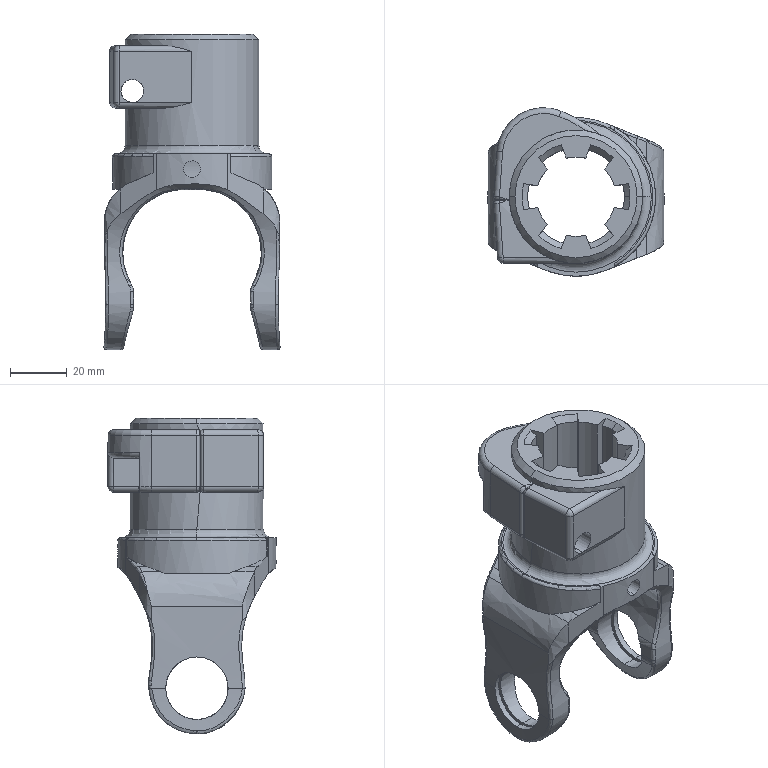Part | STEP file | CARDAN_3PARTV11 | 1 solid | 282 faces | box 61.98 x 59.195 x 111.032 mm | volume 98715 mm3 | spline 142 | cylinder 71 | plane 41 | torus 12 | cone 9 | sphere 7 | commonest cylinder face diameters 2 x18 34 x13 4 x9 22 x8 28 x6 6 x4